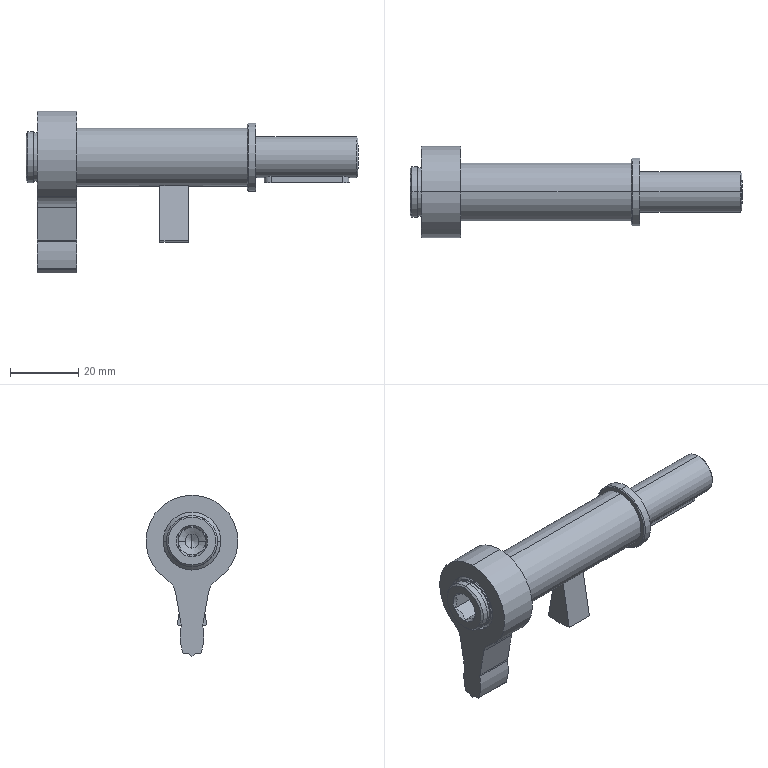Part | STEP file | PN_0033 | 1 solid | 88 faces | box 97.5 x 27 x 47.5 mm | volume 24592 mm3 | cylinder 35 | plane 33 | cone 20 | commonest cylinder face diameters 15 x4 17 x4 4 x3 1 x2 3.242 x2 4.134 x2